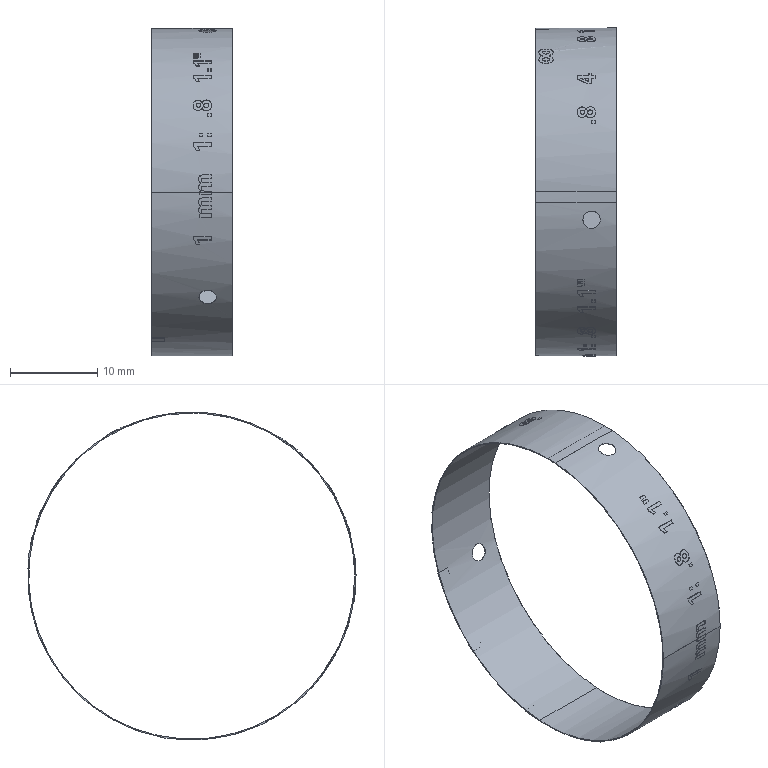Part | SolidWorks | features BaseBody 1 | 1 solid | 388 faces | box 9.2 x 37.648 x 37.599 mm | volume 107.29 mm3 | plane 180 | spline 131 | cylinder 77 | commonest cylinder face diameters 37.698 x21 37.598 x12 2 x6 3.343 x5 37.398 x4 0.566 x3